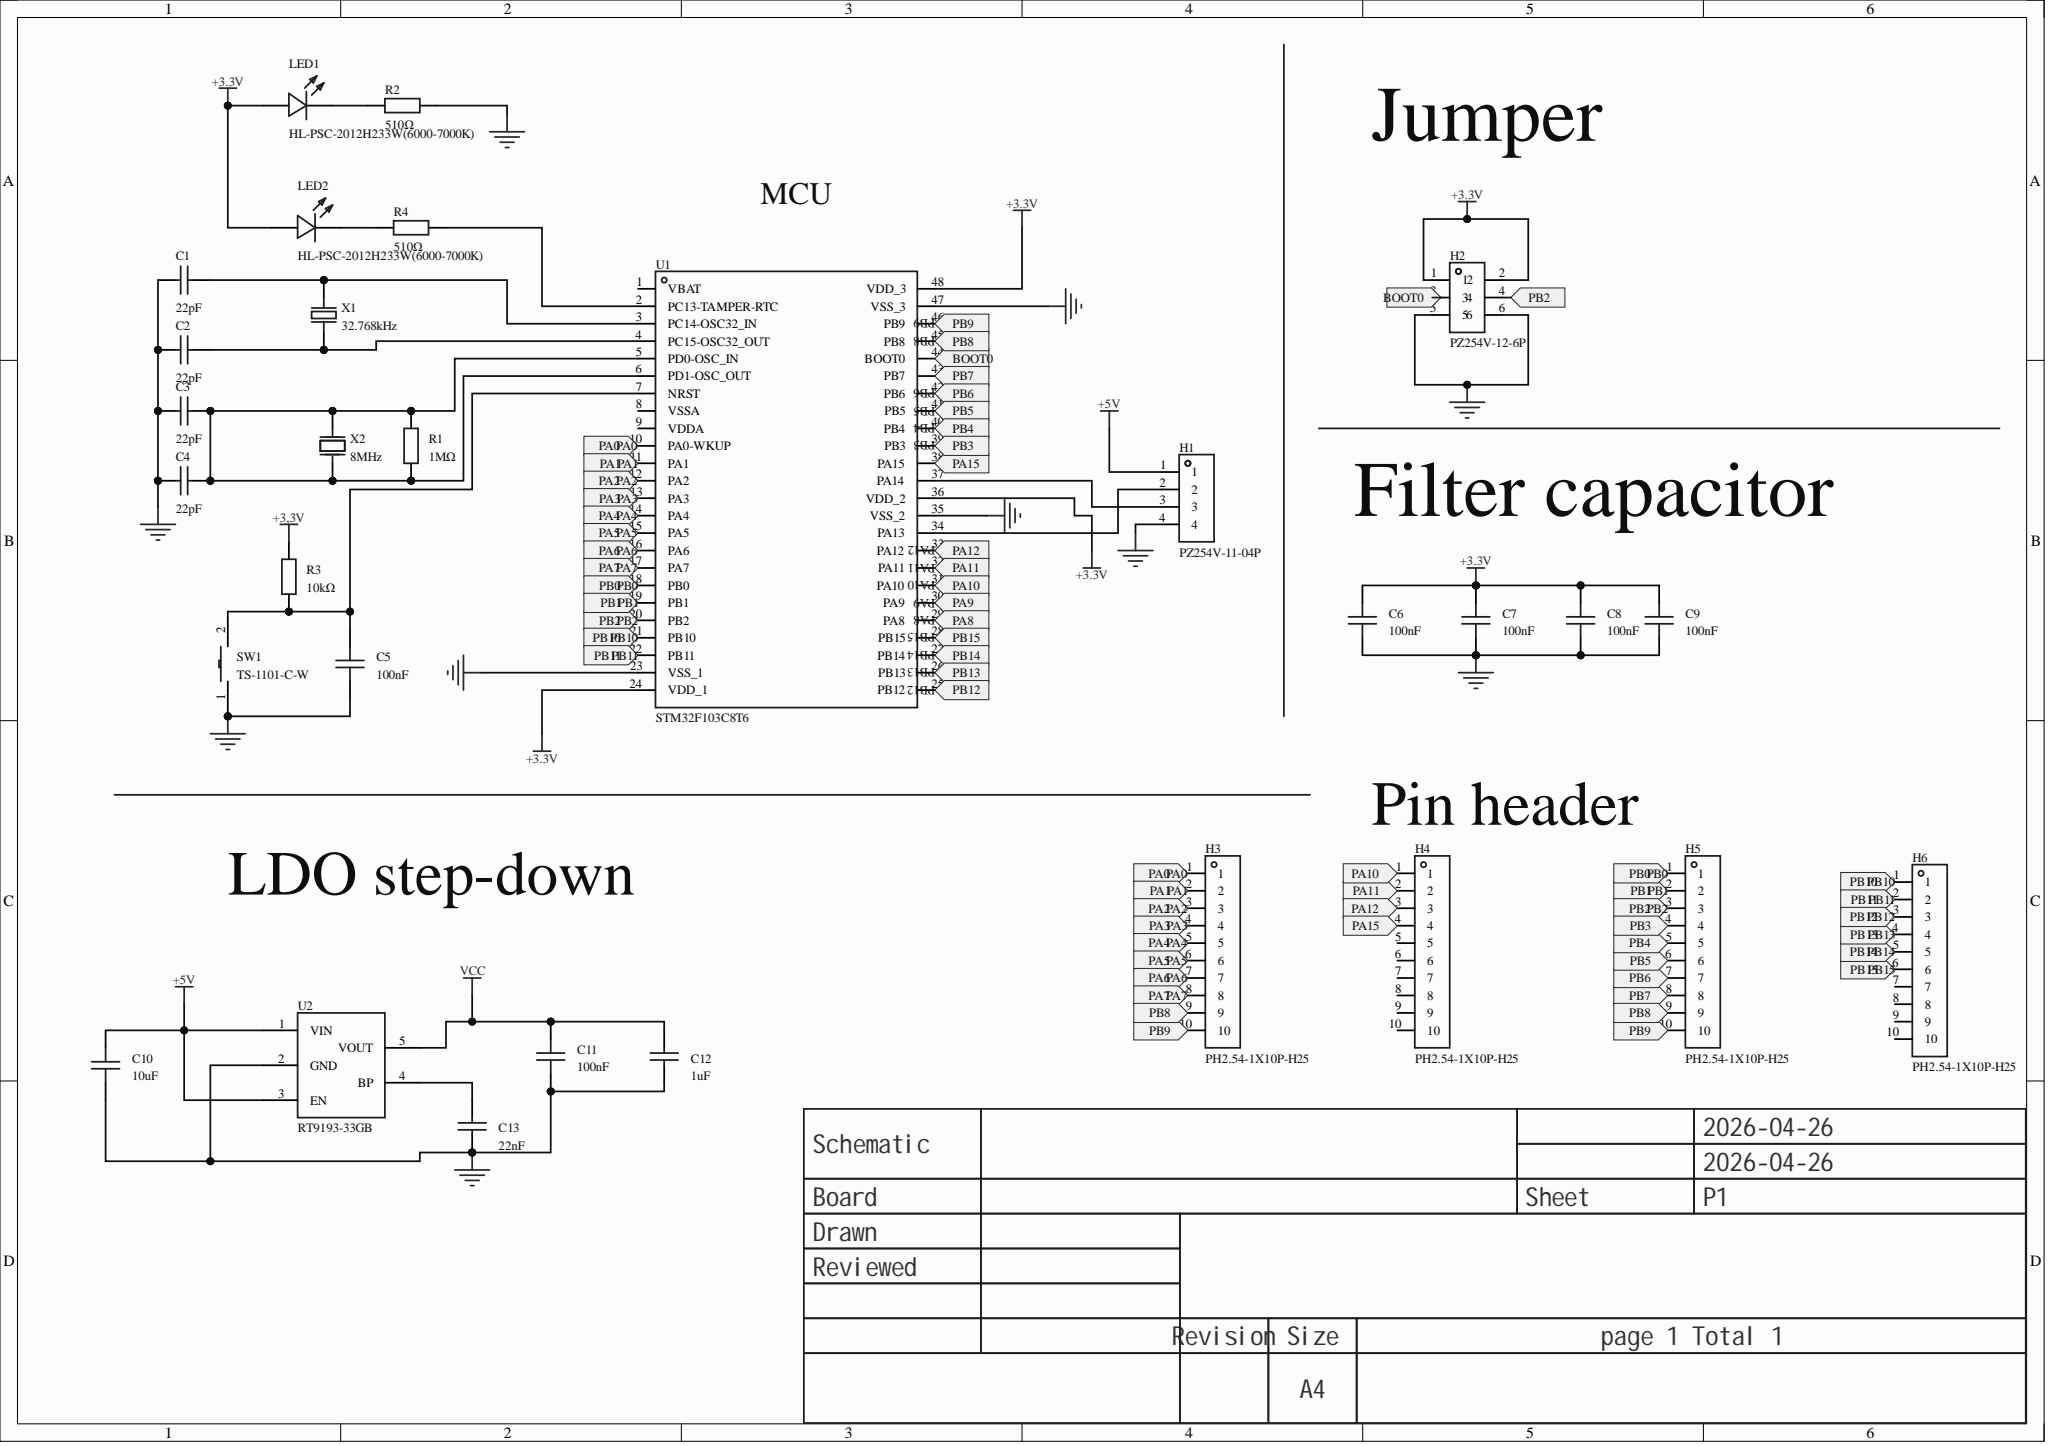Circuit board | Altium Designer | 30 parts | 43 nets
Bill of materials:
Comment,Description,Designator,Footprint,LibRef,Quantity
"22pF","Capacitance:22pF;Tolerance:±5%;Rated voltage:50V;Temperature coefficient:C0G;","C1, C2, C3, C4","C0603","CL10C220JB8NNNC","4"
"100nF","Capacitance:100nF;Tolerance:±10%;Rated voltage:50V;Temperature coefficient:X7R;","C5, C6, C7, C8, C9, C11","C0603","CC0603KRX7R9BB104","6"
"10uF","Capacitance:10uF;Tolerance:±10%;Rated voltage:10V;Temperature coefficient:X5R;","C10","C0603","CL10A106KP8NNNC","1"
"1uF","Capacitance:1uF;Tolerance:±10%;Rated voltage:16V;Temperature coefficient:X7R;","C12","C0603","CL10B105KO8NNNC","1"
"22nF","Capacitance:22nF;Tolerance:±10%;Rated voltage:50V;Temperature coefficient:X7R;","C13","C0603","CL10B223KB8NNNC","1"
"PZ254V-11-04P","Pin structure:1x4P;Pitch:2.54mm;Row spacing:-;Round/square pin:Square;Mounting:Through-hole;Rows:Single row;Total pins:4P;Rated current:3A;Rated voltage:250V;Mating pin length:6mm;Housing height:2.5mm;Termination pin length:3mm;Contact material:-;Operating temperature:-40℃~+105℃;Colour:Black;","H1","HDR-TH_4P-P2.54-V-M","PZ254V-11-04P","1"
"PZ254V-12-6P","Pin structure:2x3P;Pitch:2.54mm;Row spacing:2.54mm;Round/square pin:Square;Mounting type:Through-hole;Rows:Dual row;Total pins:6P;Rated current:-;Rated voltage:-;Mating pin length:6mm;Housing height:2.5mm;Termination pin length:3mm;Contact material:Brass;Contact plating:-;Operating temperature range:-40℃~+105℃;Colour:Black;","H2","HDR-TH_6P-P2.54-V-M-R2-C3-S2.54","PZ254V-12-6P","1"
"PH2.54-1X10P-H25","Pin structure:1x10P;Pitch:2.54mm;Row spacing:-;Round/square pin:Square;Mounting:Through-hole;Rows:Single row;Total pins:10P;Rated current:3A;Rated voltage:-;Mating pin length:6mm;Housing height:2.5mm;Termination pin length:3mm;Contact material:Brass;Contact plating:Gold;Operating temperature:-40℃~+105℃;Colour:Black;","H3, H4, H5, H6","HDR-TH_10P-P2.54-V-M","PH2.54-1X10P-H25","4"
"HL-PSC-2012H233W(6000-7000K)","Lamp base type:-;Emitting colour:White;Forward voltage (Vf):3.4V;Power:102mW;Forward current:20mA;Wavelength:-;Diode configuration:Single diode;Lens colour:Frosted yellow lens;Colour temperature:6000K~7000K;Luminous intensity:1.4cd;Viewing angle:140°;Tape packaging:Top mount;Operating temperature:-40℃~+85℃;","LED1, LED2","LED0805-R-RD","HL-PSC-2012H233W(6000-7000K)","2"
"1MΩ","Resistor type:Thick film resistor;Resistance:1MΩ;Tolerance:±1%;Power:125mW;Max working voltage:150V;Temperature coefficient:±100ppm/?;","R1","R0805","0805W8F1004T5E","1"
"510Ω","Resistor type:Thick film resistor;Resistance:510Ω;Tolerance:±1%;Power:100mW;Working voltage:75V;Temperature coefficient:±100ppm/?;","R2, R4","R0603","0603WAF5100T5E","2"
"10kΩ","Resistor type:Thick film resistor;Resistance:10kΩ;Tolerance:±1%;Power:100mW;Working voltage:75V;Temperature coefficient:±100ppm/?;","R3","R0603","0603WAF1002T5E","1"
"TS-1101-C-W","Circuit structure:SPST;Button shape:Rectangular button;Actuating force:2.6N;Mounting:Upright SMD;Switch length:6mm;Switch width:3.6mm;Switch height:2.5mm;Bracket:Without bracket;Contact current:50mA;Rated voltage:12V;Lamp:None;Life:5万 cycles;","SW1","SW-SMD_L6.0-W3.3-LS8.0_TS-1101-C-W","TS-1101-C-W","1"
"STM32F103C8T6","CPU core:ARM-M3;CPU max frequency:72MHz;Application field:-;","U1","LQFP-48_L7.0-W7.0-P0.50-LS9.0-BL","STM32F103C8T6","1"
"RT9193-33GB","Output type:Fixed;Working voltage:5.5V;Output voltage:3.3V;Output current:300mA;Power supply ripple rejection (PSRR):-50dB@(10kHz);Output polarity:Positive;","U2","SOT-23-5_L3.0-W1.7-P0.95-LS2.8-BL","RT9193-33GB","1"
"32.768kHz","Crystal type:SMD crystal;Frequency:32.768kHz;Room-temp tolerance:±20ppm;Load capacitance:12.5pF;","X1","FC-135R_L3.2-W1.5","Q13FC13500004_C32346","1"
"8MHz","Crystal type:SMD crystal;Frequency:8MHz;Room-temp tolerance:±10ppm;Load capacitance:20pF;Frequency stability:±20ppm;","X2","CRYSTAL-SMD_L5.0-W3.2","X50328MSB2GI","1"
Netlist (Protel format):
[
C1
C0603
22pF



]
[
C2
C0603
22pF



]
[
C3
C0603
22pF



]
[
C4
C0603
22pF



]
[
C5
C0603
100nF



]
[
C6
C0603
100nF



]
[
C7
C0603
100nF



]
[
C8
C0603
100nF



]
[
C9
C0603
100nF



]
[
C10
C0603
10uF



]
[
C11
C0603
100nF



]
[
C12
C0603
1uF



]
[
C13
C0603
22nF



]
[
H1
HDR-TH_4P-P2.54-V-M
PZ254V-11-04P



]
[
H2
HDR-TH_6P-P2.54-V-M-R2-C3-S2.54
PZ254V-12-6P



]
[
H3
HDR-TH_10P-P2.54-V-M
PH2.54-1X10P-H25



]
[
H4
HDR-TH_10P-P2.54-V-M
PH2.54-1X10P-H25



]
[
H5
HDR-TH_10P-P2.54-V-M
PH2.54-1X10P-H25



]
[
H6
HDR-TH_10P-P2.54-V-M
PH2.54-1X10P-H25



]
[
LED1
LED0805-R-RD
HL-PSC-2012H233W(6000-7000K)



]
[
LED2
LED0805-R-RD
HL-PSC-2012H233W(6000-7000K)



]
[
R1
R0805
1MΩ



]
[
R2
R0603
510Ω



]
[
R3
R0603
10kΩ



]
[
R4
R0603
510Ω



]
[
SW1
SW-SMD_L6.0-W3.3-LS8.0_TS-1101-C-W
TS-1101-C-W



]
[
U1
LQFP-48_L7.0-W7.0-P0.50-LS9.0-BL
STM32F103C8T6



]
[
U2
SOT-23-5_L3.0-W1.7-P0.95-LS2.8-BL
RT9193-33GB



]
[
X1
FC-135R_L3.2-W1.5
32.768kHz



]
[
X2
CRYSTAL-SMD_L5.0-W3.2
8MHz



]
(
VCC
C11-2
C12-2
U2-5
)
(
PB15
H6-6
U1-28
)
(
PB14
H6-5
U1-27
)
(
PB13
H6-4
U1-26
)
(
PB12
H6-3
U1-25
)
(
PB11
H6-2
U1-22
)
(
PB10
H6-1
U1-21
)
(
PB9
H3-10
H5-10
U1-46
)
(
PB8
H3-9
H5-9
U1-45
)
(
PB6
H5-7
U1-42
)
(
PB5
H5-6
U1-41
)
(
PB4
H5-5
U1-40
)
(
PB3
H5-4
U1-39
)
(
PB2
H2-4
H5-3
U1-20
)
(
PB1
H5-2
U1-19
)
(
PB0
H5-1
U1-18
)
(
PA12
H4-3
U1-33
)
(
PA11
H4-2
U1-32
)
(
PA10
H4-1
U1-31
)
(
PA7
H3-8
U1-17
)
(
PA6
H3-7
U1-16
)
(
PA5
H3-6
U1-15
)
(
PA4
H3-5
U1-14
)
(
PA3
H3-4
U1-13
)
(
PA2
H3-3
U1-12
)
(
PA1
H3-2
U1-11
)
(
PA0
H3-1
U1-10
)
(
NetR4_2
R4-2
U1-2
)
(
NetLED2_2
LED2-2
R4-1
)
(
NetLED1_2
LED1-2
R2-1
)
(
NetH5_8
H5-8
U1-43
)
(
NetH4_4
H4-4
U1-38
)
(
NetH2_3
H2-3
U1-44
)
(
NetH1_3
H1-3
U1-37
)
(
NetH1_2
H1-2
U1-34
)
(
NetC13_2
C13-2
U2-4
)
(
NetC5_2
C5-2
R3-1
SW1-2
U1-7
)
(
NetC3_2
C3-2
C4-2
R1-1
R1-2
U1-5
U1-6
X2-1
X2-2
)
(
NetC2_2
C2-2
U1-4
X1-1
)
(
NetC1_2
C1-2
U1-3
X1-2
)
(
GND
C1-1
C2-1
C3-1
C4-1
C5-1
C6-1
C7-1
C8-1
C9-1
C10-1
C11-1
C12-1
C13-1
H1-4
H2-5
H2-6
R2-2
SW1-1
U1-23
U1-35
U1-47
U2-2
)
(
+5V
C10-2
H1-1
U2-1
U2-3
)
(
+3.3V
C6-2
C7-2
C8-2
C9-2
H2-1
H2-2
LED1-1
LED2-1
U1-24
U1-36
U1-48
)